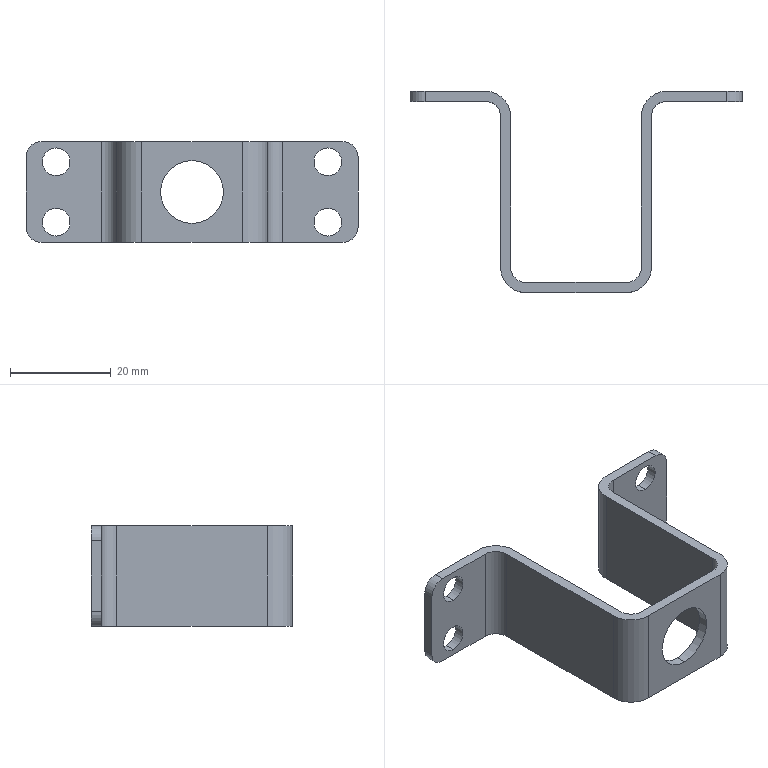Part | STEP file | Proximity mount-rotor | 1 solid | 36 faces | box 66 x 40 x 20 mm | volume 4954 mm3 | cylinder 22 | plane 14 | commonest cylinder face diameters 5.5 x8 6 x8 10 x4 12.5 x2